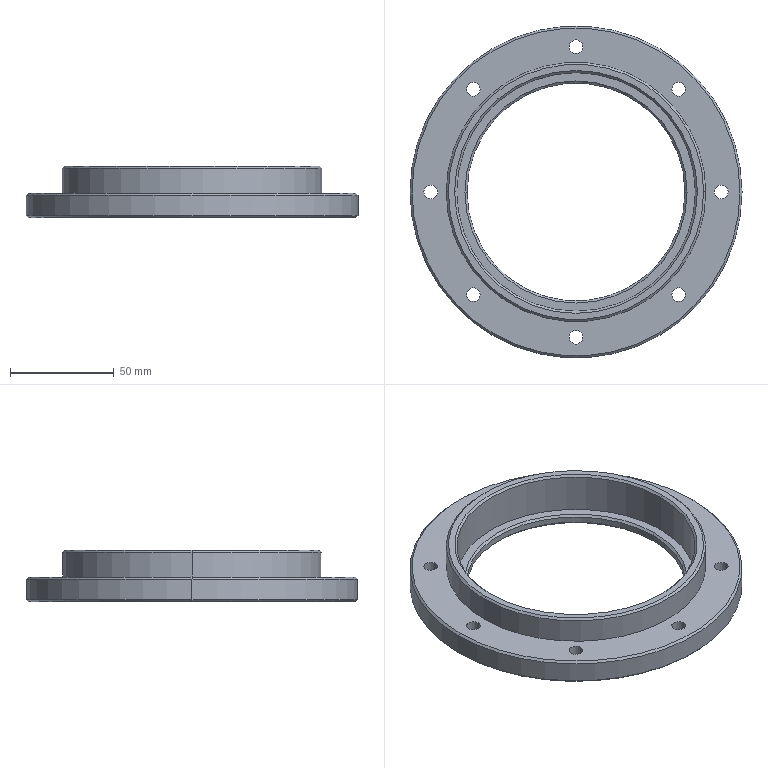Part | SolidWorks | features ICE 2, Chamfer 1, CirPattern 1, Extrusion 1, HoleWzd 1 | 1 solid | 64 faces | box 160 x 160 x 25 mm | volume 141973 mm3 | cylinder 40 | cone 12 | plane 12 | commonest cylinder face diameters 6.6 x16 11 x16 105 x2 115 x2 125 x2 160 x2